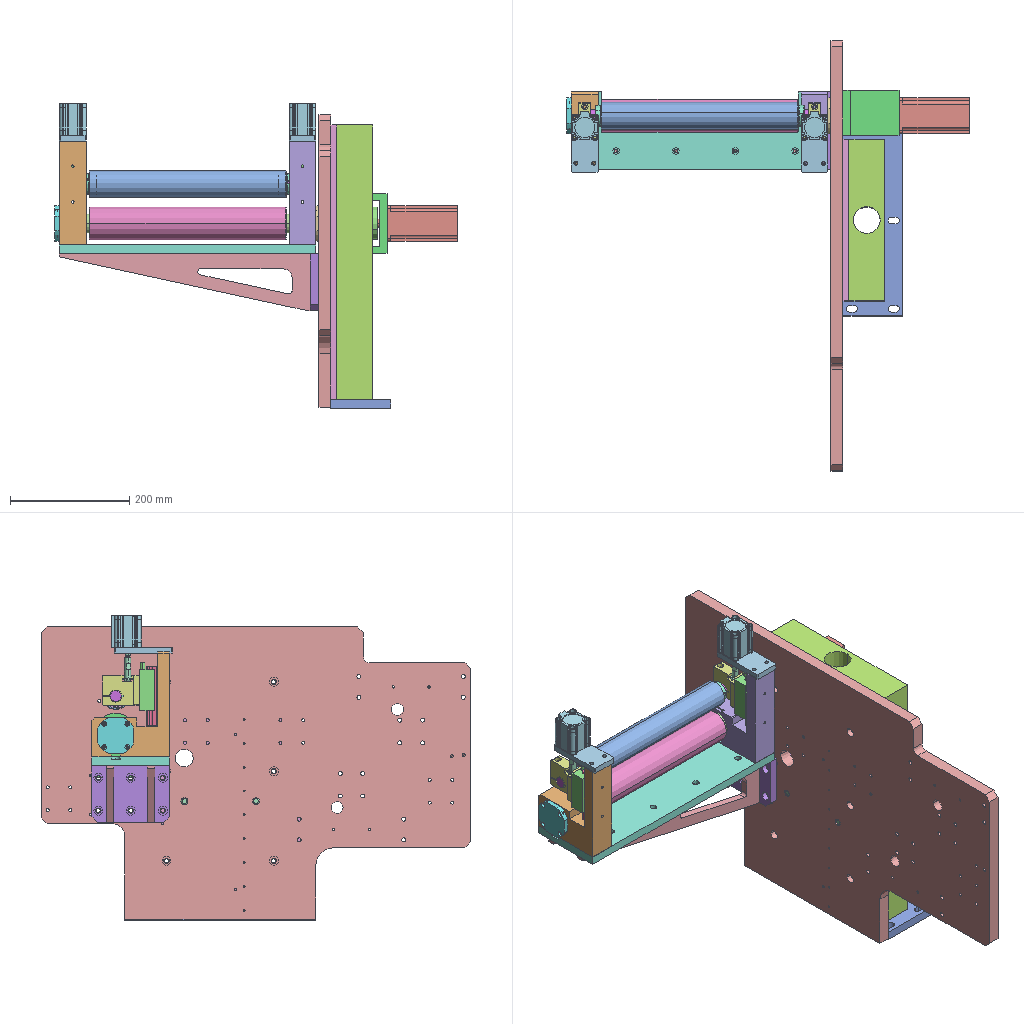Assembly | SolidWorks | 29 different items | 46 placed | box 675 x 720 x 511 mm
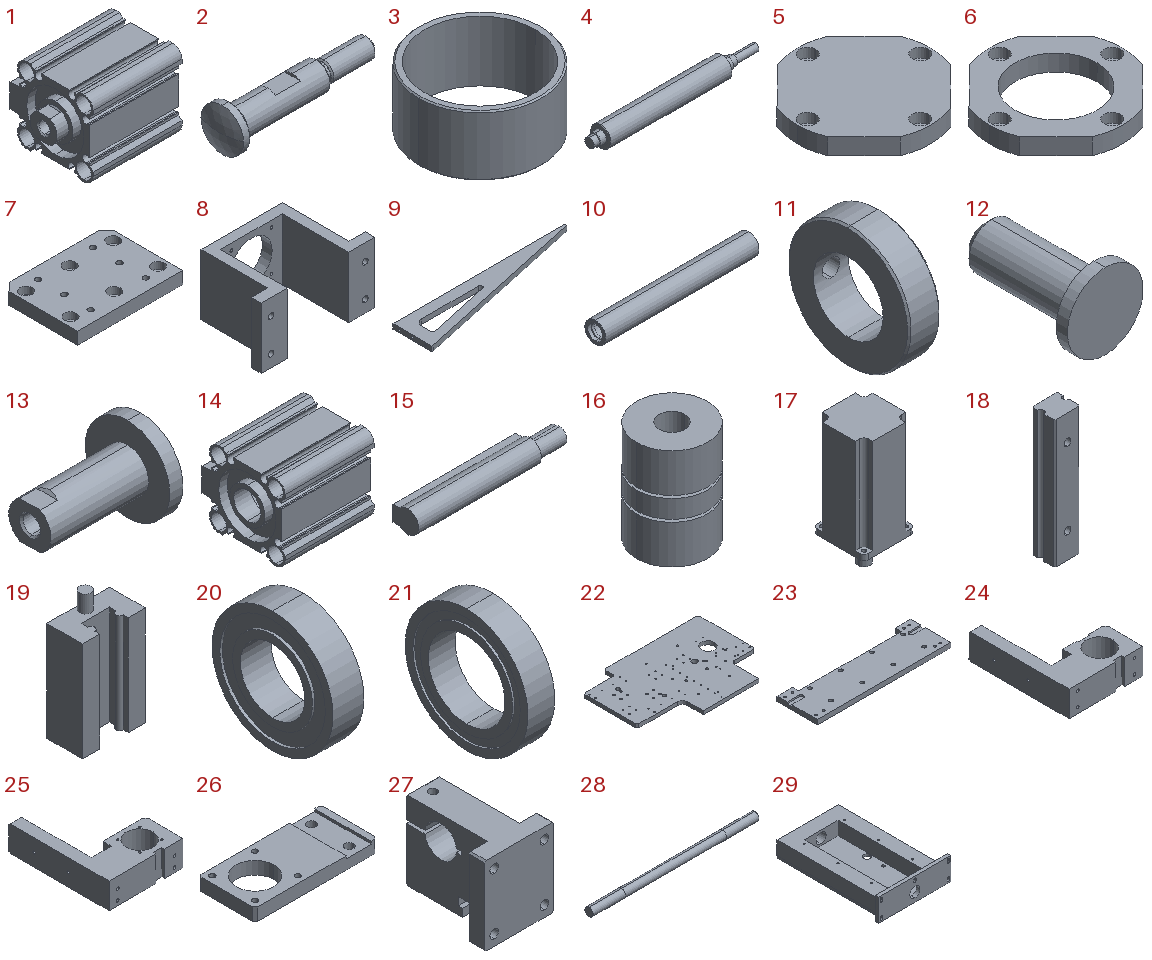Parts list (item | name | quantity | parent item | size | volume | features):
1 | (subassembly) | x2 | - | 60 x 49.5 x 45 mm | 70558 mm3 | -
2 | - | x2 | - | 59.5 x 17 x 17 mm | 5040 mm3 | features Chamfer 2, ICE 1, MirrorPattern 1, RefAxis 1, RevCut 1, Revolution 1
3 | - | x2 | - | 47 x 47 x 23 mm | 8002 mm3 | features Chamfer 1, Extrusion 1
4 | - | x1 | - | 450 x 55 x 55 mm | 841512 mm3 | features Chamfer 2, ICE 1, Revolution 1
5 | - | x1 | - | 65 x 65 x 8 mm | 24061 mm3 | features Extrusion 1, HoleWzd 1
6 | - | x1 | - | 65 x 65 x 8 mm | 14008 mm3 | features Extrusion 1, HoleWzd 1
7 | - | x1 | - | 130 x 95 x 15 mm | 166774 mm3 | features HoleWzd 2, Chamfer 1, Extrusion 1
8 | - | x1 | - | 140 x 94 x 75 mm | 246828 mm3 | features ICE 2, ExtruThin 1, HoleWzd 1
9 | - | x2 | - | 420 x 95 x 12 mm | 203565 mm3 | features HoleWzd 2, Extrusion 1
10 | - | x1 | - | 330 x 45 x 45 mm | 212984 mm3 | features ICE 4, Chamfer 1, Revolution 1
11 | - | x2 | - | 10 x 35 x 35 mm | 5795 mm3 | features 3DProfileFeature 1, Chamfer 1, HoleWzd 1, Revolution 1
12 | - | x2 | - | 20 x 32 x 20 mm | 4155 mm3 | features Chamfer 1, Revolution 1
13 | - | x2 | in 1 | 42 x 32 x 32 mm | 10910 mm3 | features RefAxis 3, 3DProfileFeature 1, ICE 1, Revolution 1
14 | - | x2 | in 1 | 53 x 49.5 x 45 mm | 58938 mm3 | features RefAxis 9, RevCut 5, 3DProfileFeature 3, Extrusion 1, ICE 1, LPattern 1
15 | - | x4 | in 1 | 27 x 4.6 x 4 mm | 354.995 mm3 | features ICE 4, RefAxis 3, 3DProfileFeature 1, Extrusion 1
16 | - | x1 | - | 55 x 55 x 78 mm | 157881 mm3 | features ICE 3, Extrusion 1
17 | - | x1 | - | 60 x 60 x 148 mm | 387738 mm3 | features ICE 3, Extrusion 1
18 | - | x2 | - | 20 x 18 x 100 mm | 32357 mm3 | features 3DProfileFeature 1, Extrusion 1, HoleWzd 1
19 | - | x2 | - | 44 x 25 x 81.8 mm | 59895 mm3 | features 3DProfileFeature 1, Extrusion 1, HoleWzd 1, ICE 1
20 | - | x2 | - | 12 x 47 x 47 mm | 13798 mm3 | features Revolution 1
21 | - | x2 | - | 7 x 32 x 32 mm | 3267 mm3 | features Revolution 1
22 | - | x1 | - | 720 x 490 x 20 mm | 5604662 mm3 | features Cut 8, HoleWzd 8, Chamfer 3, Extrusion 1, Fillet 1, ICE 1, LPattern 1
23 | - | x1 | - | 430 x 130 x 15 mm | 718358 mm3 | features HoleWzd 2, Cut 1, Extrusion 1, ICE 1
24 | - | x1 | - | 130 x 176 x 45 mm | 376408 mm3 | features HoleWzd 4, Chamfer 2, ICE 2, Extrusion 1
25 | - | x1 | - | 130 x 176 x 45 mm | 376385 mm3 | features HoleWzd 4, Chamfer 3, ICE 2, Extrusion 1
26 | - | x2 | - | 97.5 x 45 x 10 mm | 33791 mm3 | features Chamfer 1, Extrusion 1, HoleWzd 1, ICE 1
27 | - | x2 | - | 44 x 62 x 50 mm | 61273 mm3 | features HoleWzd 2, ICE 2, Chamfer 1, Extrusion 1
28 | - | x1 | - | 405 x 20 x 20 mm | 123373 mm3 | features Chamfer 1, Revolution 1
29 | - | x1 | - | 320 x 475 x 100 mm | 5416407 mm3 | features ICE 4, Cut 3, Extrusion 1, HoleWzd 1
Mates (type | each side: item.copy, entity, surface, feature):
In the top assembly
Coincident | 22.1 face plane Boss-Extrude3 | 29.1 face plane Boss-Extrude3
Coincident | 29.1 face plane Boss-Extrude4 | assembly plane
Coincident | 29.1 plane | assembly plane | 2 times
DistanceDim | 22.1 face plane Boss-Extrude3 | 29.1 face plane Boss-Extrude4
Coincident | 23.1 face plane Boss-Extrude1 | 24.1 face plane Boss-Extrude1
Concentric | 23.1 face cylinder Hole size per socket head cap screw type 0 | 24.1 face cylinder M6 Tapped Hole1
Parallel | 23.1 face plane Boss-Extrude1 | 24.1 face plane Boss-Extrude1
Coincident | 23.1 face plane Boss-Extrude1 | 25.1 face plane Boss-Extrude1
Concentric | 23.1 face cylinder Hole size per socket head cap screw type 0 | 25.1 face cylinder M6 Tapped Hole1 | 2 times
Parallel | 23.1 face plane Boss-Extrude1 | 4.1 plane
Coincident | 23.1 face plane Boss-Extrude1 | 9.1 face plane Boss-Extrude1
Coincident | 24.1 face plane Boss-Extrude1 | 18.1 face plane Extrude1
Concentric | 24.1 face cylinder M5 Tapped Hole1 | 18.1 face cylinder Hole size per socket head cap screw type 1 | 2 times
Coincident | 24.1 face plane Boss-Extrude1 | 26.1 face plane Cut-Extrude1 | 2 times
Coincident | 24.1 face plane Boss-Extrude1 | 26.1 face plane Boss-Extrude1
Concentric | 24.1 face cylinder Boss-Extrude1 | 20.1 face cylinder Revolve1
Concentric | 24.1 face cylinder Boss-Extrude1 | 3.1 face cylinder Boss-Extrude1
Coincident | 24.1 face plane Boss-Extrude1 | 3.1 face plane Boss-Extrude1
Coincident | 24.1 face plane Boss-Extrude1 | 5.1 face plane Boss-Extrude1
Concentric | 24.1 face cylinder M4 Tapped Hole1 | 5.1 face cylinder Hole size per socket head cap screw type 1 | 2 times
Coincident | 25.1 face plane Boss-Extrude1 | 18.2 face plane Extrude1
Concentric | 25.1 face cylinder M5 Tapped Hole1 | 18.2 face cylinder Hole size per socket head cap screw type 1 | 2 times
Coincident | 25.1 face plane Boss-Extrude1 | 26.2 face plane Cut-Extrude1 | 2 times
Coincident | 25.1 face plane Boss-Extrude1 | 26.2 face plane Boss-Extrude1
Concentric | 25.1 face cylinder Boss-Extrude1 | 20.2 face cylinder Revolve1
Concentric | 25.1 face cylinder Boss-Extrude1 | 3.2 face cylinder Boss-Extrude1
Concentric | 25.1 face cylinder Boss-Extrude1 | 4.1 face cylinder Boss-Extrude1
Coincident | 25.1 face plane Boss-Extrude1 | 6.1 face plane Boss-Extrude1
Concentric | 25.1 face cylinder M4 Tapped Hole1 | 6.1 face cylinder Hole size per socket head cap screw type 1 | 2 times
DistanceDim | 25.1 face plane Boss-Extrude1 | 8.1 face plane Extrude-Thin1
Parallel | 25.1 face plane Boss-Extrude1 | 8.1 face plane Extrude-Thin1
Coincident | 19.1 face plane Extrude1 | 27.1 face plane Boss-Extrude1
Concentric | 19.1 face cylinder M5 Tapped Hole1 | 27.1 face cylinder Cut-Extrude1 | 2 times
Concentric | 19.2 face cylinder Extrude1 | 18.1 face cylinder Extrude1
Coincident | 19.2 face plane Extrude1 | 27.2 face plane Boss-Extrude1
Concentric | 19.2 face cylinder M5 Tapped Hole1 | 27.2 face cylinder Cut-Extrude1 | 2 times
Concentric | 27.1 face cylinder Cut-Extrude2 | 28.1 face cylinder Revolve1
Coincident | 27.1 face plane Boss-Extrude1 | 28.1 face plane Revolve1
LimitDistanceDim | 27.1 face plane Cut-Extrude2 | 2.1 face plane Revolve1
Concentric | 27.2 face cylinder Cut-Extrude2 | 28.1 face cylinder Revolve1
Coincident | 2.1 face plane Revolve1 | 2.2 face plane Revolve1
Coincident | 20.2 face plane Revolve1 | 3.2 face plane Boss-Extrude1
Coincident | 20.2 face plane Revolve1 | 4.1 face plane Revolve1
Coincident | 20.1 face plane Revolve1 | 3.1 face plane Boss-Extrude1
Coincident | 20.1 face plane Revolve1 | 4.1 face plane Revolve1
Concentric | 4.1 face cylinder Revolve1 | 8.1 face cylinder Cut-Extrude1
Coincident | 7.1 face plane Boss-Extrude1 | 9.1 face plane Boss-Extrude1
Width | 19.1 face plane Extrude1 | 19.1 face plane Extrude1 | 18.2 face plane Extrude1 | 18.2 face plane Extrude1
Concentric | 10.1 face cylinder Revolve1 | 21.1 face cylinder Revolve1
Concentric | 10.1 face cylinder Revolve1 | 11.1 face cylinder Revolve1
Concentric | 10.1 face cylinder Revolve1 | 21.2 face cylinder Revolve1
Concentric | 10.1 face cylinder Revolve1 | 11.2 face cylinder Revolve1
Coincident | 11.2 face plane Revolve1 | 21.2 face plane Revolve1
Coincident | 11.1 face plane Revolve1 | 21.1 face plane Revolve1
Concentric | 28.1 face cylinder Revolve1 | 10.1 face cylinder Revolve1
Width | 23.1 face plane Boss-Extrude1 | 23.1 face plane Boss-Extrude1 | 11.2 face plane Revolve1 | 11.1 face plane Revolve1
Coincident | 23.1 face plane Boss-Extrude1 | 7.1 face plane Boss-Extrude1 | 2 times
Coincident | 22.1 face plane Boss-Extrude3 | 8.1 face plane Extrude-Thin1
DistanceDim | 7.1 face plane Boss-Extrude1 | 23.1 face plane Boss-Extrude1
DistanceDim | 4.1 plane | 22.1 face plane Boss-Extrude3
DistanceDim | 25.1 face plane Boss-Extrude1 | 22.1 face plane Boss-Extrude3
Concentric | 4.1 face cylinder Revolve1 | 16.1 face cylinder Boss-Extrude1
DistanceDim | 4.1 face plane Revolve1 | 16.1 face plane Boss-Extrude1
DistanceDim | 9.1 face plane Boss-Extrude1 | 7.1 face plane Boss-Extrude1
Coincident | 23.1 face plane Boss-Extrude1 | 9.2 face plane Boss-Extrude1
DistanceDim | 9.2 face plane Boss-Extrude1 | 7.1 face plane Boss-Extrude1
Coincident | 7.1 face plane Boss-Extrude1 | 9.2 face plane Boss-Extrude1
Concentric | 26.1 face cylinder Boss-Extrude1 | 13.1 face cylinder Revolve1
Coincident | 26.1 face plane Boss-Extrude1 | 14.1 face plane Boss-Extrude1
Concentric | 26.1 face cylinder M5 Tapped Hole1 | 14.1 face cylinder LPattern1
Coincident | 26.2 face plane Boss-Extrude1 | 14.2 face plane Boss-Extrude1
Concentric | 26.2 face cylinder Boss-Extrude1 | 13.2 face cylinder Revolve1
Concentric | 26.2 face cylinder M5 Tapped Hole1 | 14.2 face cylinder Cut-Revolve5
Concentric | 2.2 face cylinder Revolve1 | 13.1 face cylinder Revolve1
DistanceDim | 13.1 face plane Revolve1 | 2.2 face plane Revolve1
Coincident | 12.1 face plane Revolve1 | 12.2 face plane Revolve1
Coincident | 29.1 face plane Boss-Extrude3 | 12.1 face plane Revolve1
Concentric | 29.1 face cylinder Cut-Extrude6 | 12.1 face cylinder Revolve1
Concentric | 29.1 face cylinder Cut-Extrude6 | 12.2 face cylinder Revolve1
Coincident | 27.2 face plane Boss-Extrude1 | 28.1 face plane Revolve1
Coincident | 10.1 face plane Boss-Extrude2 | 21.1 face plane Revolve1
Coincident | 10.1 face plane Boss-Extrude1 | 21.2 face plane Revolve1
Coincident | 22.1 face plane Cut-Extrude3 | 29.1 face plane Boss-Extrude4
Concentric | 8.1 face cylinder Cut-Extrude1 | 17.1 face cylinder Extrude4
Concentric | 8.1 face cylinder M4 Tapped Hole1 | 17.1 face cylinder Extrude1
Coincident | 8.1 face plane Extrude-Thin1 | 17.1 face plane Extrude1
In subassembly 1
Coincident | 14.3 axis | 13.3 axis | 3 times
PlanarAngleDim | 13.3 plane | 14.3 plane
DistanceDim | 15.1 plane | 14.3 plane
Coincident | 14.3 axis | 15.1 axis | 3 times
PlanarAngleDim | 15.1 plane | 14.3 plane
DistanceDim | 15.2 plane | 14.3 plane
Coincident | 14.3 axis | 15.2 axis
PlanarAngleDim | 15.2 plane | 14.3 plane
LimitDistanceDim | 13.3 face plane Revolve1 | 14.3 face plane Boss-Extrude1